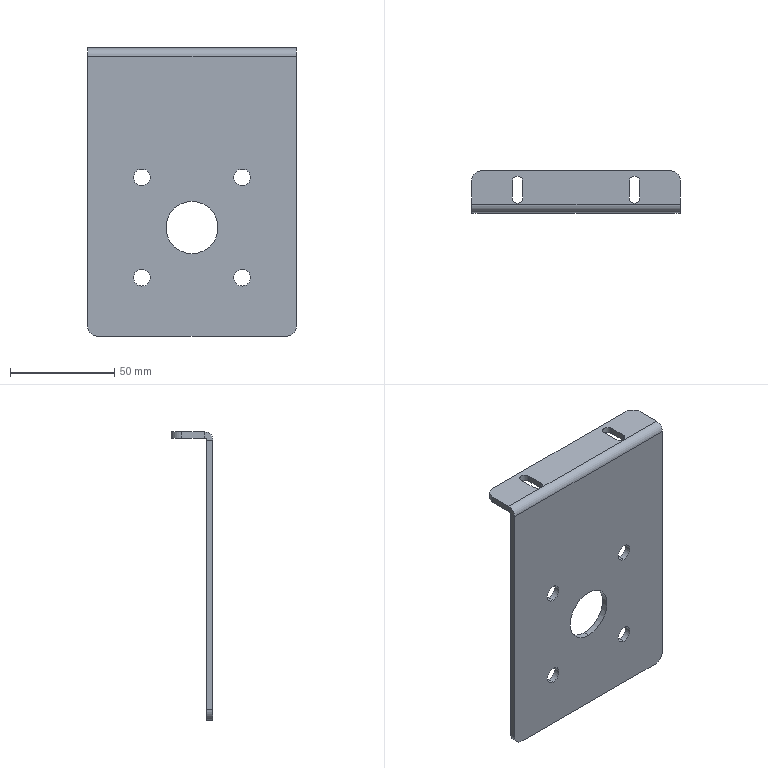Part | STEP file | 11-FG-JX00511 | 1 solid | 36 faces | box 100 x 20 x 138 mm | volume 43680 mm3 | cylinder 20 | plane 16 | commonest cylinder face diameters 8 x9 5 x4 10 x4 25 x2 2 x1
STEP:
#1=CARTESIAN_POINT('',(-24.,-10.,-66.));
#2=VERTEX_POINT('',#1);
#3=CARTESIAN_POINT('',(-24.,-10.,-58.));
#4=VERTEX_POINT('',#3);
#5=CARTESIAN_POINT('',(-24.,-10.,-62.));
#6=DIRECTION('',(0.,1.,0.));
#7=DIRECTION('',(0.,0.,1.));
#8=AXIS2_PLACEMENT_3D('',#5,#6,#7);
#9=CIRCLE('',#8,4.);
#10=EDGE_CURVE('',#2,#4,#9,.T.);
#11=ORIENTED_EDGE('',*,*,#10,.F.);
#12=CARTESIAN_POINT('',(-24.,-7.,-66.));
#13=VERTEX_POINT('',#12);
#14=CARTESIAN_POINT('',(-24.,-10.,-66.));
#15=DIRECTION('',(0.,1.,0.));
#16=VECTOR('',#15,1000.);
#17=LINE('',#14,#16);
#18=EDGE_CURVE('',#2,#13,#17,.T.);
#19=ORIENTED_EDGE('',*,*,#18,.T.);
#20=CARTESIAN_POINT('',(-24.,-7.,-58.));
#21=VERTEX_POINT('',#20);
#22=CARTESIAN_POINT('',(-24.,-7.,-62.));
#23=DIRECTION('',(0.,1.,0.));
#24=DIRECTION('',(0.,0.,1.));
#25=AXIS2_PLACEMENT_3D('',#22,#23,#24);
#26=CIRCLE('',#25,4.);
#27=EDGE_CURVE('',#13,#21,#26,.T.);
#28=ORIENTED_EDGE('',*,*,#27,.T.);
#29=CARTESIAN_POINT('',(-24.,-10.,-58.));
#30=DIRECTION('',(0.,1.,0.));
#31=VECTOR('',#30,1000.);
#32=LINE('',#29,#31);
#33=EDGE_CURVE('',#4,#21,#32,.T.);
#34=ORIENTED_EDGE('',*,*,#33,.F.);
#35=EDGE_LOOP('',(#11,#19,#28,#34));
#36=FACE_OUTER_BOUND('',#35,.T.);
#37=CARTESIAN_POINT('',(-24.,-10.,-62.));
#38=DIRECTION('',(0.,1.,0.));
#39=DIRECTION('',(0.,0.,1.));
#40=AXIS2_PLACEMENT_3D('',#37,#38,#39);
#41=CYLINDRICAL_SURFACE('',#40,4.);
#42=ADVANCED_FACE('',(#36),#41,.F.);
#43=CARTESIAN_POINT('',(-24.,-10.,-114.));
#44=VERTEX_POINT('',#43);
#45=CARTESIAN_POINT('',(-24.,-10.,-106.));
#46=VERTEX_POINT('',#45);
#47=CARTESIAN_POINT('',(-24.,-10.,-110.));
#48=DIRECTION('',(0.,1.,0.));
#49=DIRECTION('',(0.,0.,1.));
#50=AXIS2_PLACEMENT_3D('',#47,#48,#49);
#51=CIRCLE('',#50,4.);
#52=EDGE_CURVE('',#44,#46,#51,.T.);
#53=ORIENTED_EDGE('',*,*,#52,.F.);
#54=CARTESIAN_POINT('',(-24.,-7.,-114.));
#55=VERTEX_POINT('',#54);
#56=CARTESIAN_POINT('',(-24.,-10.,-114.));
#57=DIRECTION('',(0.,1.,0.));
#58=VECTOR('',#57,1000.);
#59=LINE('',#56,#58);
#60=EDGE_CURVE('',#44,#55,#59,.T.);
#61=ORIENTED_EDGE('',*,*,#60,.T.);
#62=CARTESIAN_POINT('',(-24.,-7.,-106.));
#63=VERTEX_POINT('',#62);
#64=CARTESIAN_POINT('',(-24.,-7.,-110.));
#65=DIRECTION('',(0.,1.,0.));
#66=DIRECTION('',(0.,0.,1.));
#67=AXIS2_PLACEMENT_3D('',#64,#65,#66);
#68=CIRCLE('',#67,4.);
#69=EDGE_CURVE('',#55,#63,#68,.T.);
#70=ORIENTED_EDGE('',*,*,#69,.T.);
#71=CARTESIAN_POINT('',(-24.,-10.,-106.));
#72=DIRECTION('',(0.,1.,0.));
#73=VECTOR('',#72,1000.);
#74=LINE('',#71,#73);
#75=EDGE_CURVE('',#46,#63,#74,.T.);
#76=ORIENTED_EDGE('',*,*,#75,.F.);
#77=EDGE_LOOP('',(#53,#61,#70,#76));
#78=FACE_OUTER_BOUND('',#77,.T.);
#79=CARTESIAN_POINT('',(-24.,-10.,-110.));
#80=DIRECTION('',(0.,1.,0.));
#81=DIRECTION('',(0.,0.,1.));
#82=AXIS2_PLACEMENT_3D('',#79,#80,#81);
#83=CYLINDRICAL_SURFACE('',#82,4.);
#84=ADVANCED_FACE('',(#78),#83,.F.);
#85=CARTESIAN_POINT('',(24.,-10.,-114.));
#86=VERTEX_POINT('',#85);
#87=CARTESIAN_POINT('',(24.,-10.,-106.));
#88=VERTEX_POINT('',#87);
#89=CARTESIAN_POINT('',(24.,-10.,-110.));
#90=DIRECTION('',(0.,1.,0.));
#91=DIRECTION('',(0.,0.,1.));
#92=AXIS2_PLACEMENT_3D('',#89,#90,#91);
#93=CIRCLE('',#92,4.);
#94=EDGE_CURVE('',#86,#88,#93,.T.);
#95=ORIENTED_EDGE('',*,*,#94,.F.);
#96=CARTESIAN_POINT('',(24.,-7.,-114.));
#97=VERTEX_POINT('',#96);
#98=CARTESIAN_POINT('',(24.,-10.,-114.));
#99=DIRECTION('',(0.,1.,0.));
#100=VECTOR('',#99,1000.);
#101=LINE('',#98,#100);
#102=EDGE_CURVE('',#86,#97,#101,.T.);
#103=ORIENTED_EDGE('',*,*,#102,.T.);
#104=CARTESIAN_POINT('',(24.,-7.,-106.));
#105=VERTEX_POINT('',#104);
#106=CARTESIAN_POINT('',(24.,-7.,-110.));
#107=DIRECTION('',(0.,1.,0.));
#108=DIRECTION('',(0.,0.,1.));
#109=AXIS2_PLACEMENT_3D('',#106,#107,#108);
#110=CIRCLE('',#109,4.);
#111=EDGE_CURVE('',#97,#105,#110,.T.);
#112=ORIENTED_EDGE('',*,*,#111,.T.);
#113=CARTESIAN_POINT('',(24.,-10.,-106.));
#114=DIRECTION('',(0.,1.,0.));
#115=VECTOR('',#114,1000.);
#116=LINE('',#113,#115);
#117=EDGE_CURVE('',#88,#105,#116,.T.);
#118=ORIENTED_EDGE('',*,*,#117,.F.);
#119=EDGE_LOOP('',(#95,#103,#112,#118));
#120=FACE_OUTER_BOUND('',#119,.T.);
#121=CARTESIAN_POINT('',(24.,-10.,-110.));
#122=DIRECTION('',(0.,1.,0.));
#123=DIRECTION('',(0.,0.,1.));
#124=AXIS2_PLACEMENT_3D('',#121,#122,#123);
#125=CYLINDRICAL_SURFACE('',#124,4.);
#126=ADVANCED_FACE('',(#120),#125,.F.);
#127=CARTESIAN_POINT('',(24.,-10.,-66.));
#128=VERTEX_POINT('',#127);
#129=CARTESIAN_POINT('',(24.,-10.,-58.));
#130=VERTEX_POINT('',#129);
#131=CARTESIAN_POINT('',(24.,-10.,-62.));
#132=DIRECTION('',(0.,1.,0.));
#133=DIRECTION('',(0.,0.,1.));
#134=AXIS2_PLACEMENT_3D('',#131,#132,#133);
#135=CIRCLE('',#134,4.);
#136=EDGE_CURVE('',#128,#130,#135,.T.);
#137=ORIENTED_EDGE('',*,*,#136,.F.);
#138=CARTESIAN_POINT('',(24.,-7.,-66.));
#139=VERTEX_POINT('',#138);
#140=CARTESIAN_POINT('',(24.,-10.,-66.));
#141=DIRECTION('',(0.,1.,0.));
#142=VECTOR('',#141,1000.);
#143=LINE('',#140,#142);
#144=EDGE_CURVE('',#128,#139,#143,.T.);
#145=ORIENTED_EDGE('',*,*,#144,.T.);
#146=CARTESIAN_POINT('',(24.,-7.,-58.));
#147=VERTEX_POINT('',#146);
#148=CARTESIAN_POINT('',(24.,-7.,-62.));
#149=DIRECTION('',(0.,1.,0.));
#150=DIRECTION('',(0.,0.,1.));
#151=AXIS2_PLACEMENT_3D('',#148,#149,#150);
#152=CIRCLE('',#151,4.);
#153=EDGE_CURVE('',#139,#147,#152,.T.);
#154=ORIENTED_EDGE('',*,*,#153,.T.);
#155=CARTESIAN_POINT('',(24.,-10.,-58.));
#156=DIRECTION('',(0.,1.,0.));
#157=VECTOR('',#156,1000.);
#158=LINE('',#155,#157);
#159=EDGE_CURVE('',#130,#147,#158,.T.);
#160=ORIENTED_EDGE('',*,*,#159,.F.);
#161=EDGE_LOOP('',(#137,#145,#154,#160));
#162=FACE_OUTER_BOUND('',#161,.T.);
#163=CARTESIAN_POINT('',(24.,-10.,-62.));
#164=DIRECTION('',(0.,1.,0.));
#165=DIRECTION('',(0.,0.,1.));
#166=AXIS2_PLACEMENT_3D('',#163,#164,#165);
#167=CYLINDRICAL_SURFACE('',#166,4.);
#168=ADVANCED_FACE('',(#162),#167,.F.);
#169=CARTESIAN_POINT('',(0.,-10.,-98.5));
#170=VERTEX_POINT('',#169);
#171=CARTESIAN_POINT('',(0.,-10.,-73.5));
#172=VERTEX_POINT('',#171);
#173=CARTESIAN_POINT('',(0.,-10.,-86.));
#174=DIRECTION('',(0.,1.,0.));
#175=DIRECTION('',(0.,0.,1.));
#176=AXIS2_PLACEMENT_3D('',#173,#174,#175);
#177=CIRCLE('',#176,12.5);
#178=EDGE_CURVE('',#170,#172,#177,.T.);
#179=ORIENTED_EDGE('',*,*,#178,.F.);
#180=CARTESIAN_POINT('',(0.,-7.,-98.5));
#181=VERTEX_POINT('',#180);
#182=CARTESIAN_POINT('',(0.,-10.,-98.5));
#183=DIRECTION('',(0.,1.,0.));
#184=VECTOR('',#183,1000.);
#185=LINE('',#182,#184);
#186=EDGE_CURVE('',#170,#181,#185,.T.);
#187=ORIENTED_EDGE('',*,*,#186,.T.);
#188=CARTESIAN_POINT('',(0.,-7.,-73.5));
#189=VERTEX_POINT('',#188);
#190=CARTESIAN_POINT('',(0.,-7.,-86.));
#191=DIRECTION('',(0.,1.,0.));
#192=DIRECTION('',(0.,0.,1.));
#193=AXIS2_PLACEMENT_3D('',#190,#191,#192);
#194=CIRCLE('',#193,12.5);
#195=EDGE_CURVE('',#181,#189,#194,.T.);
#196=ORIENTED_EDGE('',*,*,#195,.T.);
#197=CARTESIAN_POINT('',(0.,-10.,-73.5));
#198=DIRECTION('',(0.,1.,0.));
#199=VECTOR('',#198,1000.);
#200=LINE('',#197,#199);
#201=EDGE_CURVE('',#172,#189,#200,.T.);
#202=ORIENTED_EDGE('',*,*,#201,.F.);
#203=EDGE_LOOP('',(#179,#187,#196,#202));
#204=FACE_OUTER_BOUND('',#203,.T.);
#205=CARTESIAN_POINT('',(0.,-10.,-86.));
#206=DIRECTION('',(0.,1.,0.));
#207=DIRECTION('',(0.,0.,1.));
#208=AXIS2_PLACEMENT_3D('',#205,#206,#207);
#209=CYLINDRICAL_SURFACE('',#208,12.5);
#210=ADVANCED_FACE('',(#204),#209,.F.);
#211=CARTESIAN_POINT('',(-50.,5.,0.));
#212=VERTEX_POINT('',#211);
#213=CARTESIAN_POINT('',(-50.,-6.,0.));
#214=VERTEX_POINT('',#213);
#215=CARTESIAN_POINT('',(-50.,10.,0.));
#216=DIRECTION('',(0.,-1.,0.));
#217=VECTOR('',#216,1000.);
#218=LINE('',#215,#217);
#219=EDGE_CURVE('',#212,#214,#218,.T.);
#220=ORIENTED_EDGE('',*,*,#219,.F.);
#221=CARTESIAN_POINT('',(-50.,5.,-3.));
#222=VERTEX_POINT('',#221);
#223=CARTESIAN_POINT('',(-50.,5.,-3.));
#224=DIRECTION('',(0.,0.,-1.));
#225=VECTOR('',#224,1000.);
#226=LINE('',#223,#225);
#227=EDGE_CURVE('',#212,#222,#226,.T.);
#228=ORIENTED_EDGE('',*,*,#227,.T.);
#229=CARTESIAN_POINT('',(-50.,-6.,-3.));
#230=VERTEX_POINT('',#229);
#231=CARTESIAN_POINT('',(-50.,10.,-3.));
#232=DIRECTION('',(0.,-1.,0.));
#233=VECTOR('',#232,1000.);
#234=LINE('',#231,#233);
#235=EDGE_CURVE('',#222,#230,#234,.T.);
#236=ORIENTED_EDGE('',*,*,#235,.T.);
#237=CARTESIAN_POINT('',(-50.,-6.,-3.));
#238=DIRECTION('',(0.,0.,1.));
#239=VECTOR('',#238,1000.);
#240=LINE('',#237,#239);
#241=EDGE_CURVE('',#230,#214,#240,.T.);
#242=ORIENTED_EDGE('',*,*,#241,.T.);
#243=EDGE_LOOP('',(#220,#228,#236,#242));
#244=FACE_OUTER_BOUND('',#243,.T.);
#245=CARTESIAN_POINT('',(-50.,10.,-3.));
#246=DIRECTION('',(-1.,0.,0.));
#247=DIRECTION('',(0.,0.,1.));
#248=AXIS2_PLACEMENT_3D('',#245,#246,#247);
#249=PLANE('',#248);
#250=ADVANCED_FACE('',(#244),#249,.T.);
#251=CARTESIAN_POINT('',(30.5,5.,-3.));
#252=VERTEX_POINT('',#251);
#253=CARTESIAN_POINT('',(30.5,-3.,-3.));
#254=VERTEX_POINT('',#253);
#255=CARTESIAN_POINT('',(30.5,5.,-3.));
#256=DIRECTION('',(0.,-1.,0.));
#257=VECTOR('',#256,1000.);
#258=LINE('',#255,#257);
#259=EDGE_CURVE('',#252,#254,#258,.T.);
#260=ORIENTED_EDGE('',*,*,#259,.F.);
#261=CARTESIAN_POINT('',(25.5,5.,-3.));
#262=VERTEX_POINT('',#261);
#263=CARTESIAN_POINT('',(28.,5.,-3.));
#264=DIRECTION('',(0.,0.,-1.));
#265=DIRECTION('',(1.,0.,0.));
#266=AXIS2_PLACEMENT_3D('',#263,#264,#265);
#267=CIRCLE('',#266,2.5);
#268=EDGE_CURVE('',#262,#252,#267,.T.);
#269=ORIENTED_EDGE('',*,*,#268,.F.);
#270=CARTESIAN_POINT('',(25.5,-3.,-3.));
#271=VERTEX_POINT('',#270);
#272=CARTESIAN_POINT('',(25.5,5.,-3.));
#273=DIRECTION('',(0.,1.,0.));
#274=VECTOR('',#273,1000.);
#275=LINE('',#272,#274);
#276=EDGE_CURVE('',#271,#262,#275,.T.);
#277=ORIENTED_EDGE('',*,*,#276,.F.);
#278=CARTESIAN_POINT('',(28.,-3.,-3.));
#279=DIRECTION('',(0.,0.,-1.));
#280=DIRECTION('',(1.,0.,0.));
#281=AXIS2_PLACEMENT_3D('',#278,#279,#280);
#282=CIRCLE('',#281,2.5);
#283=EDGE_CURVE('',#254,#271,#282,.T.);
#284=ORIENTED_EDGE('',*,*,#283,.F.);
#285=EDGE_LOOP('',(#260,#269,#277,#284));
#286=FACE_BOUND('',#285,.T.);
#287=CARTESIAN_POINT('',(-25.5,5.,-3.));
#288=VERTEX_POINT('',#287);
#289=CARTESIAN_POINT('',(-25.5,-3.,-3.));
#290=VERTEX_POINT('',#289);
#291=CARTESIAN_POINT('',(-25.5,5.,-3.));
#292=DIRECTION('',(0.,-1.,0.));
#293=VECTOR('',#292,1000.);
#294=LINE('',#291,#293);
#295=EDGE_CURVE('',#288,#290,#294,.T.);
#296=ORIENTED_EDGE('',*,*,#295,.F.);
#297=CARTESIAN_POINT('',(-30.5,5.,-3.));
#298=VERTEX_POINT('',#297);
#299=CARTESIAN_POINT('',(-28.,5.,-3.));
#300=DIRECTION('',(0.,0.,-1.));
#301=DIRECTION('',(-1.,0.,0.));
#302=AXIS2_PLACEMENT_3D('',#299,#300,#301);
#303=CIRCLE('',#302,2.5);
#304=EDGE_CURVE('',#298,#288,#303,.T.);
#305=ORIENTED_EDGE('',*,*,#304,.F.);
#306=CARTESIAN_POINT('',(-30.5,-3.,-3.));
#307=VERTEX_POINT('',#306);
#308=CARTESIAN_POINT('',(-30.5,5.,-3.));
#309=DIRECTION('',(0.,1.,0.));
#310=VECTOR('',#309,1000.);
#311=LINE('',#308,#310);
#312=EDGE_CURVE('',#307,#298,#311,.T.);
#313=ORIENTED_EDGE('',*,*,#312,.F.);
#314=CARTESIAN_POINT('',(-28.,-3.,-3.));
#315=DIRECTION('',(0.,0.,-1.));
#316=DIRECTION('',(-1.,0.,0.));
#317=AXIS2_PLACEMENT_3D('',#314,#315,#316);
#318=CIRCLE('',#317,2.5);
#319=EDGE_CURVE('',#290,#307,#318,.T.);
#320=ORIENTED_EDGE('',*,*,#319,.F.);
#321=EDGE_LOOP('',(#296,#305,#313,#320));
#322=FACE_BOUND('',#321,.T.);
#323=CARTESIAN_POINT('',(45.,10.,-3.));
#324=VERTEX_POINT('',#323);
#325=CARTESIAN_POINT('',(-45.,10.,-3.));
#326=VERTEX_POINT('',#325);
#327=CARTESIAN_POINT('',(-50.,10.,-3.));
#328=DIRECTION('',(-1.,0.,0.));
#329=VECTOR('',#328,1000.);
#330=LINE('',#327,#329);
#331=EDGE_CURVE('',#324,#326,#330,.T.);
#332=ORIENTED_EDGE('',*,*,#331,.F.);
#333=CARTESIAN_POINT('',(50.,5.,-3.));
#334=VERTEX_POINT('',#333);
#335=CARTESIAN_POINT('',(45.,5.,-3.));
#336=DIRECTION('',(0.,0.,-1.));
#337=DIRECTION('',(1.,0.,0.));
#338=AXIS2_PLACEMENT_3D('',#335,#336,#337);
#339=CIRCLE('',#338,5.);
#340=EDGE_CURVE('',#324,#334,#339,.T.);
#341=ORIENTED_EDGE('',*,*,#340,.T.);
#342=CARTESIAN_POINT('',(50.,-6.,-3.));
#343=VERTEX_POINT('',#342);
#344=CARTESIAN_POINT('',(50.,10.,-3.));
#345=DIRECTION('',(0.,1.,0.));
#346=VECTOR('',#345,1000.);
#347=LINE('',#344,#346);
#348=EDGE_CURVE('',#343,#334,#347,.T.);
#349=ORIENTED_EDGE('',*,*,#348,.F.);
#350=CARTESIAN_POINT('',(-50.,-6.,-3.));
#351=DIRECTION('',(1.,0.,0.));
#352=VECTOR('',#351,1000.);
#353=LINE('',#350,#352);
#354=EDGE_CURVE('',#230,#343,#353,.T.);
#355=ORIENTED_EDGE('',*,*,#354,.F.);
#356=ORIENTED_EDGE('',*,*,#235,.F.);
#357=CARTESIAN_POINT('',(-45.,5.,-3.));
#358=DIRECTION('',(0.,0.,-1.));
#359=DIRECTION('',(1.,0.,0.));
#360=AXIS2_PLACEMENT_3D('',#357,#358,#359);
#361=CIRCLE('',#360,5.);
#362=EDGE_CURVE('',#222,#326,#361,.T.);
#363=ORIENTED_EDGE('',*,*,#362,.T.);
#364=EDGE_LOOP('',(#332,#341,#349,#355,#356,#363));
#365=FACE_OUTER_BOUND('',#364,.T.);
#366=CARTESIAN_POINT('',(0.,0.,-3.));
#367=DIRECTION('',(0.,0.,1.));
#368=DIRECTION('',(1.,0.,0.));
#369=AXIS2_PLACEMENT_3D('',#366,#367,#368);
#370=PLANE('',#369);
#371=ADVANCED_FACE('',(#286,#322,#365),#370,.F.);
#372=CARTESIAN_POINT('',(25.5,5.,0.));
#373=VERTEX_POINT('',#372);
#374=CARTESIAN_POINT('',(30.5,5.,0.));
#375=VERTEX_POINT('',#374);
#376=CARTESIAN_POINT('',(28.,5.,0.));
#377=DIRECTION('',(0.,0.,-1.));
#378=DIRECTION('',(1.,0.,0.));
#379=AXIS2_PLACEMENT_3D('',#376,#377,#378);
#380=CIRCLE('',#379,2.5);
#381=EDGE_CURVE('',#373,#375,#380,.T.);
#382=ORIENTED_EDGE('',*,*,#381,.T.);
#383=CARTESIAN_POINT('',(30.5,-3.,0.));
#384=VERTEX_POINT('',#383);
#385=CARTESIAN_POINT('',(30.5,5.,0.));
#386=DIRECTION('',(0.,-1.,0.));
#387=VECTOR('',#386,1000.);
#388=LINE('',#385,#387);
#389=EDGE_CURVE('',#375,#384,#388,.T.);
#390=ORIENTED_EDGE('',*,*,#389,.T.);
#391=CARTESIAN_POINT('',(25.5,-3.,0.));
#392=VERTEX_POINT('',#391);
#393=CARTESIAN_POINT('',(28.,-3.,0.));
#394=DIRECTION('',(0.,0.,-1.));
#395=DIRECTION('',(1.,0.,0.));
#396=AXIS2_PLACEMENT_3D('',#393,#394,#395);
#397=CIRCLE('',#396,2.5);
#398=EDGE_CURVE('',#384,#392,#397,.T.);
#399=ORIENTED_EDGE('',*,*,#398,.T.);
#400=CARTESIAN_POINT('',(25.5,5.,0.));
#401=DIRECTION('',(0.,1.,0.));
#402=VECTOR('',#401,1000.);
#403=LINE('',#400,#402);
#404=EDGE_CURVE('',#392,#373,#403,.T.);
#405=ORIENTED_EDGE('',*,*,#404,.T.);
#406=EDGE_LOOP('',(#382,#390,#399,#405));
#407=FACE_BOUND('',#406,.T.);
#408=CARTESIAN_POINT('',(-30.5,5.,0.));
#409=VERTEX_POINT('',#408);
#410=CARTESIAN_POINT('',(-25.5,5.,0.));
#411=VERTEX_POINT('',#410);
#412=CARTESIAN_POINT('',(-28.,5.,0.));
#413=DIRECTION('',(0.,0.,-1.));
#414=DIRECTION('',(-1.,0.,0.));
#415=AXIS2_PLACEMENT_3D('',#412,#413,#414);
#416=CIRCLE('',#415,2.5);
#417=EDGE_CURVE('',#409,#411,#416,.T.);
#418=ORIENTED_EDGE('',*,*,#417,.T.);
#419=CARTESIAN_POINT('',(-25.5,-3.,0.));
#420=VERTEX_POINT('',#419);
#421=CARTESIAN_POINT('',(-25.5,5.,0.));
#422=DIRECTION('',(0.,-1.,0.));
#423=VECTOR('',#422,1000.);
#424=LINE('',#421,#423);
#425=EDGE_CURVE('',#411,#420,#424,.T.);
#426=ORIENTED_EDGE('',*,*,#425,.T.);
#427=CARTESIAN_POINT('',(-30.5,-3.,0.));
#428=VERTEX_POINT('',#427);
#429=CARTESIAN_POINT('',(-28.,-3.,0.));
#430=DIRECTION('',(0.,0.,-1.));
#431=DIRECTION('',(-1.,0.,0.));
#432=AXIS2_PLACEMENT_3D('',#429,#430,#431);
#433=CIRCLE('',#432,2.5);
#434=EDGE_CURVE('',#420,#428,#433,.T.);
#435=ORIENTED_EDGE('',*,*,#434,.T.);
#436=CARTESIAN_POINT('',(-30.5,5.,0.));
#437=DIRECTION('',(0.,1.,0.));
#438=VECTOR('',#437,1000.);
#439=LINE('',#436,#438);
#440=EDGE_CURVE('',#428,#409,#439,.T.);
#441=ORIENTED_EDGE('',*,*,#440,.T.);
#442=EDGE_LOOP('',(#418,#426,#435,#441));
#443=FACE_BOUND('',#442,.T.);
#444=CARTESIAN_POINT('',(50.,-6.,0.));
#445=VERTEX_POINT('',#444);
#446=CARTESIAN_POINT('',(50.,5.,0.));
#447=VERTEX_POINT('',#446);
#448=CARTESIAN_POINT('',(50.,10.,0.));
#449=DIRECTION('',(0.,1.,0.));
#450=VECTOR('',#449,1000.);
#451=LINE('',#448,#450);
#452=EDGE_CURVE('',#445,#447,#451,.T.);
#453=ORIENTED_EDGE('',*,*,#452,.T.);
#454=CARTESIAN_POINT('',(45.,10.,0.));
#455=VERTEX_POINT('',#454);
#456=CARTESIAN_POINT('',(45.,5.,0.));
#457=DIRECTION('',(0.,0.,1.));
#458=DIRECTION('',(1.,0.,0.));
#459=AXIS2_PLACEMENT_3D('',#456,#457,#458);
#460=CIRCLE('',#459,5.);
#461=EDGE_CURVE('',#447,#455,#460,.T.);
#462=ORIENTED_EDGE('',*,*,#461,.T.);
#463=CARTESIAN_POINT('',(-45.,10.,0.));
#464=VERTEX_POINT('',#463);
#465=CARTESIAN_POINT('',(-50.,10.,0.));
#466=DIRECTION('',(-1.,0.,0.));
#467=VECTOR('',#466,1000.);
#468=LINE('',#465,#467);
#469=EDGE_CURVE('',#455,#464,#468,.T.);
#470=ORIENTED_EDGE('',*,*,#469,.T.);
#471=CARTESIAN_POINT('',(-45.,5.,0.));
#472=DIRECTION('',(0.,0.,1.));
#473=DIRECTION('',(1.,0.,0.));
#474=AXIS2_PLACEMENT_3D('',#471,#472,#473);
#475=CIRCLE('',#474,5.);
#476=EDGE_CURVE('',#464,#212,#475,.T.);
#477=ORIENTED_EDGE('',*,*,#476,.T.);
#478=ORIENTED_EDGE('',*,*,#219,.T.);
#479=CARTESIAN_POINT('',(-50.,-6.,0.));
#480=DIRECTION('',(1.,0.,0.));
#481=VECTOR('',#480,1000.);
#482=LINE('',#479,#481);
#483=EDGE_CURVE('',#214,#445,#482,.T.);
#484=ORIENTED_EDGE('',*,*,#483,.T.);
#485=EDGE_LOOP('',(#453,#462,#470,#477,#478,#484));
#486=FACE_OUTER_BOUND('',#485,.T.);
#487=CARTESIAN_POINT('',(0.,0.,0.));
#488=DIRECTION('',(0.,0.,1.));
#489=DIRECTION('',(1.,0.,0.));
#490=AXIS2_PLACEMENT_3D('',#487,#488,#489);
#491=PLANE('',#490);
#492=ADVANCED_FACE('',(#407,#443,#486),#491,.T.);
#493=ORIENTED_EDGE('',*,*,#348,.T.);
#494=CARTESIAN_POINT('',(50.,5.,-3.));
#495=DIRECTION('',(0.,0.,1.));
#496=VECTOR('',#495,1000.);
#497=LINE('',#494,#496);
#498=EDGE_CURVE('',#334,#447,#497,.T.);
#499=ORIENTED_EDGE('',*,*,#498,.T.);
#500=ORIENTED_EDGE('',*,*,#452,.F.);
#501=CARTESIAN_POINT('',(50.,-6.,-3.));
#502=DIRECTION('',(0.,0.,1.));
#503=VECTOR('',#502,1000.);
#504=LINE('',#501,#503);
#505=EDGE_CURVE('',#343,#445,#504,.T.);
#506=ORIENTED_EDGE('',*,*,#505,.F.);
#507=EDGE_LOOP('',(#493,#499,#500,#506));
#508=FACE_OUTER_BOUND('',#507,.T.);
#509=CARTESIAN_POINT('',(50.,10.,-3.));
#510=DIRECTION('',(1.,0.,0.));
#511=DIRECTION('',(0.,1.,0.));
#512=AXIS2_PLACEMENT_3D('',#509,#510,#511);
#513=PLANE('',#512);
#514=ADVANCED_FACE('',(#508),#513,.T.);
#515=ORIENTED_EDGE('',*,*,#469,.F.);
#516=CARTESIAN_POINT('',(45.,10.,-3.));
#517=DIRECTION('',(0.,0.,-1.));
#518=VECTOR('',#517,1000.);
#519=LINE('',#516,#518);
#520=EDGE_CURVE('',#455,#324,#519,.T.);
#521=ORIENTED_EDGE('',*,*,#520,.T.);
#522=ORIENTED_EDGE('',*,*,#331,.T.);
#523=CARTESIAN_POINT('',(-45.,10.,-3.));
#524=DIRECTION('',(0.,0.,1.));
#525=VECTOR('',#524,1000.);
#526=LINE('',#523,#525);
#527=EDGE_CURVE('',#326,#464,#526,.T.);
#528=ORIENTED_EDGE('',*,*,#527,.T.);
#529=EDGE_LOOP('',(#515,#521,#522,#528));
#530=FACE_OUTER_BOUND('',#529,.T.);
#531=CARTESIAN_POINT('',(-50.,10.,-3.));
#532=DIRECTION('',(0.,1.,0.));
#533=DIRECTION('',(0.,0.,1.));
#534=AXIS2_PLACEMENT_3D('',#531,#532,#533);
#535=PLANE('',#534);
#536=ADVANCED_FACE('',(#530),#535,.T.);
#537=CARTESIAN_POINT('',(50.,-7.,-4.));
#538=VERTEX_POINT('',#537);
#539=CARTESIAN_POINT('',(50.,-10.,-4.));
#540=VERTEX_POINT('',#539);
#541=CARTESIAN_POINT('',(50.,-10.,-4.));
#542=DIRECTION('',(0.,-1.,0.));
#543=VECTOR('',#542,1000.);
#544=LINE('',#541,#543);
#545=EDGE_CURVE('',#538,#540,#544,.T.);
#546=ORIENTED_EDGE('',*,*,#545,.F.);
#547=CARTESIAN_POINT('',(50.,-6.,-4.));
#548=DIRECTION('',(1.,0.,0.));
#549=DIRECTION('',(0.,0.,1.));
#550=AXIS2_PLACEMENT_3D('',#547,#548,#549);
#551=CIRCLE('',#550,1.);
#552=EDGE_CURVE('',#343,#538,#551,.T.);
#553=ORIENTED_EDGE('',*,*,#552,.F.);
#554=ORIENTED_EDGE('',*,*,#505,.T.);
#555=CARTESIAN_POINT('',(50.,-6.,-4.));
#556=DIRECTION('',(1.,0.,0.));
#557=DIRECTION('',(0.,0.,1.));
#558=AXIS2_PLACEMENT_3D('',#555,#556,#557);
#559=CIRCLE('',#558,4.);
#560=EDGE_CURVE('',#445,#540,#559,.T.);
#561=ORIENTED_EDGE('',*,*,#560,.T.);
#562=EDGE_LOOP('',(#546,#553,#554,#561));
#563=FACE_OUTER_BOUND('',#562,.T.);
#564=CARTESIAN_POINT('',(50.,-6.,-4.));
#565=DIRECTION('',(1.,0.,0.));
#566=DIRECTION('',(0.,0.,-1.));
#567=AXIS2_PLACEMENT_3D('',#564,#565,#566);
#568=PLANE('',#567);
#569=ADVANCED_FACE('',(#563),#568,.T.);
#570=CARTESIAN_POINT('',(-50.,-7.,-4.));
#571=VERTEX_POINT('',#570);
#572=CARTESIAN_POINT('',(-50.,-6.,-4.));
#573=DIRECTION('',(-1.,0.,0.));
#574=DIRECTION('',(0.,0.,1.));
#575=AXIS2_PLACEMENT_3D('',#572,#573,#574);
#576=CIRCLE('',#575,1.);
#577=EDGE_CURVE('',#571,#230,#576,.T.);
#578=ORIENTED_EDGE('',*,*,#577,.F.);
#579=CARTESIAN_POINT('',(-50.,-10.,-4.));
#580=VERTEX_POINT('',#579);
#581=CARTESIAN_POINT('',(-50.,-7.,-4.));
#582=DIRECTION('',(0.,-1.,0.));
#583=VECTOR('',#582,1000.);
#584=LINE('',#581,#583);
#585=EDGE_CURVE('',#571,#580,#584,.T.);
#586=ORIENTED_EDGE('',*,*,#585,.T.);
#587=CARTESIAN_POINT('',(-50.,-6.,-4.));
#588=DIRECTION('',(-1.,0.,0.));
#589=DIRECTION('',(0.,0.,1.));
#590=AXIS2_PLACEMENT_3D('',#587,#588,#589);
#591=CIRCLE('',#590,4.);
#592=EDGE_CURVE('',#580,#214,#591,.T.);
#593=ORIENTED_EDGE('',*,*,#592,.T.);
#594=ORIENTED_EDGE('',*,*,#241,.F.);
#595=EDGE_LOOP('',(#578,#586,#593,#594));
#596=FACE_OUTER_BOUND('',#595,.T.);
#597=CARTESIAN_POINT('',(-50.,-6.,-4.));
#598=DIRECTION('',(1.,0.,0.));
#599=DIRECTION('',(0.,0.,-1.));
#600=AXIS2_PLACEMENT_3D('',#597,#598,#599);
#601=PLANE('',#600);
#602=ADVANCED_FACE('',(#596),#601,.F.);
#603=ORIENTED_EDGE('',*,*,#483,.F.);
#604=ORIENTED_EDGE('',*,*,#592,.F.);
#605=CARTESIAN_POINT('',(50.,-10.,-4.));
#606=DIRECTION('',(1.,0.,0.));
#607=VECTOR('',#606,1000.);
#608=LINE('',#605,#607);
#609=EDGE_CURVE('',#580,#540,#608,.T.);
#610=ORIENTED_EDGE('',*,*,#609,.T.);
#611=ORIENTED_EDGE('',*,*,#560,.F.);
#612=EDGE_LOOP('',(#603,#604,#610,#611));
#613=FACE_OUTER_BOUND('',#612,.T.);
#614=CARTESIAN_POINT('',(-50.,-6.,-4.));
#615=DIRECTION('',(-1.,0.,0.));
#616=DIRECTION('',(0.,-1.,0.));
#617=AXIS2_PLACEMENT_3D('',#614,#615,#616);
#618=CYLINDRICAL_SURFACE('',#617,4.);
#619=ADVANCED_FACE('',(#613),#618,.T.);
#620=ORIENTED_EDGE('',*,*,#354,.T.);
#621=ORIENTED_EDGE('',*,*,#552,.T.);
#622=CARTESIAN_POINT('',(50.,-7.,-4.));
#623=DIRECTION('',(-1.,0.,0.));
#624=VECTOR('',#623,1000.);
#625=LINE('',#622,#624);
#626=EDGE_CURVE('',#538,#571,#625,.T.);
#627=ORIENTED_EDGE('',*,*,#626,.T.);
#628=ORIENTED_EDGE('',*,*,#577,.T.);
#629=EDGE_LOOP('',(#620,#621,#627,#628));
#630=FACE_OUTER_BOUND('',#629,.T.);
#631=CARTESIAN_POINT('',(-50.,-6.,-4.));
#632=DIRECTION('',(-1.,0.,0.));
#633=DIRECTION('',(0.,-1.,0.));
#634=AXIS2_PLACEMENT_3D('',#631,#632,#633);
#635=CYLINDRICAL_SURFACE('',#634,1.);
#636=ADVANCED_FACE('',(#630),#635,.F.);
#637=CARTESIAN_POINT('',(-50.,-7.,-133.));
#638=VERTEX_POINT('',#637);
#639=CARTESIAN_POINT('',(-50.,-7.,-138.));
#640=DIRECTION('',(0.,0.,-1.));
#641=VECTOR('',#640,1000.);
#642=LINE('',#639,#641);
#643=EDGE_CURVE('',#571,#638,#642,.T.);
#644=ORIENTED_EDGE('',*,*,#643,.T.);
#645=CARTESIAN_POINT('',(-50.,-10.,-133.));
#646=VERTEX_POINT('',#645);
#647=CARTESIAN_POINT('',(-50.,-10.,-133.));
#648=DIRECTION('',(0.,-1.,0.));
#649=VECTOR('',#648,1000.);
#650=LINE('',#647,#649);
#651=EDGE_CURVE('',#638,#646,#650,.T.);
#652=ORIENTED_EDGE('',*,*,#651,.T.);
#653=CARTESIAN_POINT('',(-50.,-10.,0.));
#654=DIRECTION('',(0.,0.,-1.));
#655=VECTOR('',#654,1000.);
#656=LINE('',#653,#655);
#657=EDGE_CURVE('',#580,#646,#656,.T.);
#658=ORIENTED_EDGE('',*,*,#657,.F.);
#659=ORIENTED_EDGE('',*,*,#585,.F.);
#660=EDGE_LOOP('',(#644,#652,#658,#659));
#661=FACE_OUTER_BOUND('',#660,.T.);
#662=CARTESIAN_POINT('',(-50.,-10.,-138.));
#663=DIRECTION('',(1.,0.,0.));
#664=DIRECTION('',(0.,0.,-1.));
#665=AXIS2_PLACEMENT_3D('',#662,#663,#664);
#666=PLANE('',#665);
#667=ADVANCED_FACE('',(#661),#666,.F.);
#668=CARTESIAN_POINT('',(50.,-10.,-133.));
#669=VERTEX_POINT('',#668);
#670=CARTESIAN_POINT('',(50.,-10.,0.));
#671=DIRECTION('',(0.,0.,1.));
#672=VECTOR('',#671,1000.);
#673=LINE('',#670,#672);
#674=EDGE_CURVE('',#669,#540,#673,.T.);
#675=ORIENTED_EDGE('',*,*,#674,.F.);
#676=CARTESIAN_POINT('',(50.,-7.,-133.));
#677=VERTEX_POINT('',#676);
#678=CARTESIAN_POINT('',(50.,-10.,-133.));
#679=DIRECTION('',(0.,1.,0.));
#680=VECTOR('',#679,1000.);
#681=LINE('',#678,#680);
#682=EDGE_CURVE('',#669,#677,#681,.T.);
#683=ORIENTED_EDGE('',*,*,#682,.T.);
#684=CARTESIAN_POINT('',(50.,-7.,-3.));
#685=DIRECTION('',(0.,0.,1.));
#686=VECTOR('',#685,1000.);
#687=LINE('',#684,#686);
#688=EDGE_CURVE('',#677,#538,#687,.T.);
#689=ORIENTED_EDGE('',*,*,#688,.T.);
#690=ORIENTED_EDGE('',*,*,#545,.T.);
#691=EDGE_LOOP('',(#675,#683,#689,#690));
#692=FACE_OUTER_BOUND('',#691,.T.);
#693=CARTESIAN_POINT('',(50.,-10.,-3.));
#694=DIRECTION('',(-1.,0.,0.));
#695=DIRECTION('',(0.,0.,1.));
#696=AXIS2_PLACEMENT_3D('',#693,#694,#695);
#697=PLANE('',#696);
#698=ADVANCED_FACE('',(#692),#697,.F.);
#699=CARTESIAN_POINT('',(-24.,-10.,-62.));
#700=DIRECTION('',(0.,1.,0.));
#701=DIRECTION('',(0.,0.,1.));
#702=AXIS2_PLACEMENT_3D('',#699,#700,#701);
#703=CIRCLE('',#702,4.);
#704=EDGE_CURVE('',#4,#2,#703,.T.);
#705=ORIENTED_EDGE('',*,*,#704,.T.);
#706=ORIENTED_EDGE('',*,*,#10,.T.);
#707=EDGE_LOOP('',(#705,#706));
#708=FACE_BOUND('',#707,.T.);
#709=CARTESIAN_POINT('',(-24.,-10.,-110.));
#710=DIRECTION('',(0.,1.,0.));
#711=DIRECTION('',(0.,0.,1.));
#712=AXIS2_PLACEMENT_3D('',#709,#710,#711);
#713=CIRCLE('',#712,4.);
#714=EDGE_CURVE('',#46,#44,#713,.T.);
#715=ORIENTED_EDGE('',*,*,#714,.T.);
#716=ORIENTED_EDGE('',*,*,#52,.T.);
#717=EDGE_LOOP('',(#715,#716));
#718=FACE_BOUND('',#717,.T.);
#719=CARTESIAN_POINT('',(24.,-10.,-110.));
#720=DIRECTION('',(0.,1.,0.));
#721=DIRECTION('',(0.,0.,1.));
#722=AXIS2_PLACEMENT_3D('',#719,#720,#721);
#723=CIRCLE('',#722,4.);
#724=EDGE_CURVE('',#88,#86,#723,.T.);
#725=ORIENTED_EDGE('',*,*,#724,.T.);
#726=ORIENTED_EDGE('',*,*,#94,.T.);
#727=EDGE_LOOP('',(#725,#726));
#728=FACE_BOUND('',#727,.T.);
#729=CARTESIAN_POINT('',(24.,-10.,-62.));
#730=DIRECTION('',(0.,1.,0.));
#731=DIRECTION('',(0.,0.,1.));
#732=AXIS2_PLACEMENT_3D('',#729,#730,#731);
#733=CIRCLE('',#732,4.);
#734=EDGE_CURVE('',#130,#128,#733,.T.);
#735=ORIENTED_EDGE('',*,*,#734,.T.);
#736=ORIENTED_EDGE('',*,*,#136,.T.);
#737=EDGE_LOOP('',(#735,#736));
#738=FACE_BOUND('',#737,.T.);
#739=CARTESIAN_POINT('',(0.,-10.,-86.));
#740=DIRECTION('',(0.,1.,0.));
#741=DIRECTION('',(0.,0.,1.));
#742=AXIS2_PLACEMENT_3D('',#739,#740,#741);
#743=CIRCLE('',#742,12.5);
#744=EDGE_CURVE('',#172,#170,#743,.T.);
#745=ORIENTED_EDGE('',*,*,#744,.T.);
#746=ORIENTED_EDGE('',*,*,#178,.T.);
#747=EDGE_LOOP('',(#745,#746));
#748=FACE_BOUND('',#747,.T.);
#749=CARTESIAN_POINT('',(-45.,-10.,-138.));
#750=VERTEX_POINT('',#749);
#751=CARTESIAN_POINT('',(45.,-10.,-138.));
#752=VERTEX_POINT('',#751);
#753=CARTESIAN_POINT('',(0.,-10.,-138.));
#754=DIRECTION('',(1.,0.,0.));
#755=VECTOR('',#754,1000.);
#756=LINE('',#753,#755);
#757=EDGE_CURVE('',#750,#752,#756,.T.);
#758=ORIENTED_EDGE('',*,*,#757,.T.);
#759=CARTESIAN_POINT('',(45.,-10.,-133.));
#760=DIRECTION('',(0.,-1.,0.));
#761=DIRECTION('',(0.,0.,1.));
#762=AXIS2_PLACEMENT_3D('',#759,#760,#761);
#763=CIRCLE('',#762,5.);
#764=EDGE_CURVE('',#752,#669,#763,.T.);
#765=ORIENTED_EDGE('',*,*,#764,.T.);
#766=ORIENTED_EDGE('',*,*,#674,.T.);
#767=ORIENTED_EDGE('',*,*,#609,.F.);
#768=ORIENTED_EDGE('',*,*,#657,.T.);
#769=CARTESIAN_POINT('',(-45.,-10.,-133.));
#770=DIRECTION('',(0.,-1.,0.));
#771=DIRECTION('',(0.,0.,1.));
#772=AXIS2_PLACEMENT_3D('',#769,#770,#771);
#773=CIRCLE('',#772,5.);
#774=EDGE_CURVE('',#646,#750,#773,.T.);
#775=ORIENTED_EDGE('',*,*,#774,.T.);
#776=EDGE_LOOP('',(#758,#765,#766,#767,#768,#775));
#777=FACE_OUTER_BOUND('',#776,.T.);
#778=CARTESIAN_POINT('',(0.,-10.,0.));
#779=DIRECTION('',(0.,1.,0.));
#780=DIRECTION('',(0.,0.,1.));
#781=AXIS2_PLACEMENT_3D('',#778,#779,#780);
#782=PLANE('',#781);
#783=ADVANCED_FACE('',(#708,#718,#728,#738,#748,#777),#782,.F.);
#784=CARTESIAN_POINT('',(-24.,-7.,-62.));
#785=DIRECTION('',(0.,1.,0.));
#786=DIRECTION('',(0.,0.,1.));
#787=AXIS2_PLACEMENT_3D('',#784,#785,#786);
#788=CIRCLE('',#787,4.);
#789=EDGE_CURVE('',#21,#13,#788,.T.);
#790=ORIENTED_EDGE('',*,*,#789,.F.);
#791=ORIENTED_EDGE('',*,*,#27,.F.);
#792=EDGE_LOOP('',(#790,#791));
#793=FACE_BOUND('',#792,.T.);
#794=CARTESIAN_POINT('',(-24.,-7.,-110.));
#795=DIRECTION('',(0.,1.,0.));
#796=DIRECTION('',(0.,0.,1.));
#797=AXIS2_PLACEMENT_3D('',#794,#795,#796);
#798=CIRCLE('',#797,4.);
#799=EDGE_CURVE('',#63,#55,#798,.T.);
#800=ORIENTED_EDGE('',*,*,#799,.F.);
#801=ORIENTED_EDGE('',*,*,#69,.F.);
#802=EDGE_LOOP('',(#800,#801));
#803=FACE_BOUND('',#802,.T.);
#804=CARTESIAN_POINT('',(24.,-7.,-110.));
#805=DIRECTION('',(0.,1.,0.));
#806=DIRECTION('',(0.,0.,1.));
#807=AXIS2_PLACEMENT_3D('',#804,#805,#806);
#808=CIRCLE('',#807,4.);
#809=EDGE_CURVE('',#105,#97,#808,.T.);
#810=ORIENTED_EDGE('',*,*,#809,.F.);
#811=ORIENTED_EDGE('',*,*,#111,.F.);
#812=EDGE_LOOP('',(#810,#811));
#813=FACE_BOUND('',#812,.T.);
#814=CARTESIAN_POINT('',(24.,-7.,-62.));
#815=DIRECTION('',(0.,1.,0.));
#816=DIRECTION('',(0.,0.,1.));
#817=AXIS2_PLACEMENT_3D('',#814,#815,#816);
#818=CIRCLE('',#817,4.);
#819=EDGE_CURVE('',#147,#139,#818,.T.);
#820=ORIENTED_EDGE('',*,*,#819,.F.);
#821=ORIENTED_EDGE('',*,*,#153,.F.);
#822=EDGE_LOOP('',(#820,#821));
#823=FACE_BOUND('',#822,.T.);
#824=CARTESIAN_POINT('',(0.,-7.,-86.));
#825=DIRECTION('',(0.,1.,0.));
#826=DIRECTION('',(0.,0.,1.));
#827=AXIS2_PLACEMENT_3D('',#824,#825,#826);
#828=CIRCLE('',#827,12.5);
#829=EDGE_CURVE('',#189,#181,#828,.T.);
#830=ORIENTED_EDGE('',*,*,#829,.F.);
#831=ORIENTED_EDGE('',*,*,#195,.F.);
#832=EDGE_LOOP('',(#830,#831));
#833=FACE_BOUND('',#832,.T.);
#834=ORIENTED_EDGE('',*,*,#688,.F.);
#835=CARTESIAN_POINT('',(45.,-7.,-138.));
#836=VERTEX_POINT('',#835);
#837=CARTESIAN_POINT('',(45.,-7.,-133.));
#838=DIRECTION('',(0.,1.,0.));
#839=DIRECTION('',(0.,0.,1.));
#840=AXIS2_PLACEMENT_3D('',#837,#838,#839);
#841=CIRCLE('',#840,5.);
#842=EDGE_CURVE('',#677,#836,#841,.T.);
#843=ORIENTED_EDGE('',*,*,#842,.T.);
#844=CARTESIAN_POINT('',(-45.,-7.,-138.));
#845=VERTEX_POINT('',#844);
#846=CARTESIAN_POINT('',(50.,-7.,-138.));
#847=DIRECTION('',(1.,0.,0.));
#848=VECTOR('',#847,1000.);
#849=LINE('',#846,#848);
#850=EDGE_CURVE('',#845,#836,#849,.T.);
#851=ORIENTED_EDGE('',*,*,#850,.F.);
#852=CARTESIAN_POINT('',(-45.,-7.,-133.));
#853=DIRECTION('',(0.,1.,0.));
#854=DIRECTION('',(0.,0.,1.));
#855=AXIS2_PLACEMENT_3D('',#852,#853,#854);
#856=CIRCLE('',#855,5.);
#857=EDGE_CURVE('',#845,#638,#856,.T.);
#858=ORIENTED_EDGE('',*,*,#857,.T.);
#859=ORIENTED_EDGE('',*,*,#643,.F.);
#860=ORIENTED_EDGE('',*,*,#626,.F.);
#861=EDGE_LOOP('',(#834,#843,#851,#858,#859,#860));
#862=FACE_OUTER_BOUND('',#861,.T.);
#863=CARTESIAN_POINT('',(0.,-7.,0.));
#864=DIRECTION('',(0.,1.,0.));
#865=DIRECTION('',(0.,0.,1.));
#866=AXIS2_PLACEMENT_3D('',#863,#864,#865);
#867=PLANE('',#866);
#868=ADVANCED_FACE('',(#793,#803,#813,#823,#833,#862),#867,.T.);
#869=ORIENTED_EDGE('',*,*,#850,.T.);
#870=CARTESIAN_POINT('',(45.,-10.,-138.));
#871=DIRECTION('',(0.,-1.,0.));
#872=VECTOR('',#871,1000.);
#873=LINE('',#870,#872);
#874=EDGE_CURVE('',#836,#752,#873,.T.);
#875=ORIENTED_EDGE('',*,*,#874,.T.);
#876=ORIENTED_EDGE('',*,*,#757,.F.);
#877=CARTESIAN_POINT('',(-45.,-10.,-138.));
#878=DIRECTION('',(0.,1.,0.));
#879=VECTOR('',#878,1000.);
#880=LINE('',#877,#879);
#881=EDGE_CURVE('',#750,#845,#880,.T.);
#882=ORIENTED_EDGE('',*,*,#881,.T.);
#883=EDGE_LOOP('',(#869,#875,#876,#882));
#884=FACE_OUTER_BOUND('',#883,.T.);
#885=CARTESIAN_POINT('',(50.,-10.,-138.));
#886=DIRECTION('',(0.,0.,1.));
#887=DIRECTION('',(0.,-1.,0.));
#888=AXIS2_PLACEMENT_3D('',#885,#886,#887);
#889=PLANE('',#888);
#890=ADVANCED_FACE('',(#884),#889,.F.);
#891=ORIENTED_EDGE('',*,*,#186,.F.);
#892=ORIENTED_EDGE('',*,*,#744,.F.);
#893=ORIENTED_EDGE('',*,*,#201,.T.);
#894=ORIENTED_EDGE('',*,*,#829,.T.);
#895=EDGE_LOOP('',(#891,#892,#893,#894));
#896=FACE_OUTER_BOUND('',#895,.T.);
#897=CARTESIAN_POINT('',(0.,-10.,-86.));
#898=DIRECTION('',(0.,1.,0.));
#899=DIRECTION('',(0.,0.,1.));
#900=AXIS2_PLACEMENT_3D('',#897,#898,#899);
#901=CYLINDRICAL_SURFACE('',#900,12.5);
#902=ADVANCED_FACE('',(#896),#901,.F.);
#903=ORIENTED_EDGE('',*,*,#144,.F.);
#904=ORIENTED_EDGE('',*,*,#734,.F.);
#905=ORIENTED_EDGE('',*,*,#159,.T.);
#906=ORIENTED_EDGE('',*,*,#819,.T.);
#907=EDGE_LOOP('',(#903,#904,#905,#906));
#908=FACE_OUTER_BOUND('',#907,.T.);
#909=CARTESIAN_POINT('',(24.,-10.,-62.));
#910=DIRECTION('',(0.,1.,0.));
#911=DIRECTION('',(0.,0.,1.));
#912=AXIS2_PLACEMENT_3D('',#909,#910,#911);
#913=CYLINDRICAL_SURFACE('',#912,4.);
#914=ADVANCED_FACE('',(#908),#913,.F.);
#915=ORIENTED_EDGE('',*,*,#102,.F.);
#916=ORIENTED_EDGE('',*,*,#724,.F.);
#917=ORIENTED_EDGE('',*,*,#117,.T.);
#918=ORIENTED_EDGE('',*,*,#809,.T.);
#919=EDGE_LOOP('',(#915,#916,#917,#918));
#920=FACE_OUTER_BOUND('',#919,.T.);
#921=CARTESIAN_POINT('',(24.,-10.,-110.));
#922=DIRECTION('',(0.,1.,0.));
#923=DIRECTION('',(0.,0.,1.));
#924=AXIS2_PLACEMENT_3D('',#921,#922,#923);
#925=CYLINDRICAL_SURFACE('',#924,4.);
#926=ADVANCED_FACE('',(#920),#925,.F.);
#927=ORIENTED_EDGE('',*,*,#60,.F.);
#928=ORIENTED_EDGE('',*,*,#714,.F.);
#929=ORIENTED_EDGE('',*,*,#75,.T.);
#930=ORIENTED_EDGE('',*,*,#799,.T.);
#931=EDGE_LOOP('',(#927,#928,#929,#930));
#932=FACE_OUTER_BOUND('',#931,.T.);
#933=CARTESIAN_POINT('',(-24.,-10.,-110.));
#934=DIRECTION('',(0.,1.,0.));
#935=DIRECTION('',(0.,0.,1.));
#936=AXIS2_PLACEMENT_3D('',#933,#934,#935);
#937=CYLINDRICAL_SURFACE('',#936,4.);
#938=ADVANCED_FACE('',(#932),#937,.F.);
#939=ORIENTED_EDGE('',*,*,#18,.F.);
#940=ORIENTED_EDGE('',*,*,#704,.F.);
#941=ORIENTED_EDGE('',*,*,#33,.T.);
#942=ORIENTED_EDGE('',*,*,#789,.T.);
#943=EDGE_LOOP('',(#939,#940,#941,#942));
#944=FACE_OUTER_BOUND('',#943,.T.);
#945=CARTESIAN_POINT('',(-24.,-10.,-62.));
#946=DIRECTION('',(0.,1.,0.));
#947=DIRECTION('',(0.,0.,1.));
#948=AXIS2_PLACEMENT_3D('',#945,#946,#947);
#949=CYLINDRICAL_SURFACE('',#948,4.);
#950=ADVANCED_FACE('',(#944),#949,.F.);
#951=ORIENTED_EDGE('',*,*,#304,.T.);
#952=CARTESIAN_POINT('',(-25.5,5.,0.));
#953=DIRECTION('',(0.,0.,-1.));
#954=VECTOR('',#953,1000.);
#955=LINE('',#952,#954);
#956=EDGE_CURVE('',#411,#288,#955,.T.);
#957=ORIENTED_EDGE('',*,*,#956,.F.);
#958=ORIENTED_EDGE('',*,*,#417,.F.);
#959=CARTESIAN_POINT('',(-30.5,5.,0.));
#960=DIRECTION('',(0.,0.,-1.));
#961=VECTOR('',#960,1000.);
#962=LINE('',#959,#961);
#963=EDGE_CURVE('',#409,#298,#962,.T.);
#964=ORIENTED_EDGE('',*,*,#963,.T.);
#965=EDGE_LOOP('',(#951,#957,#958,#964));
#966=FACE_OUTER_BOUND('',#965,.T.);
#967=CARTESIAN_POINT('',(-28.,5.,0.));
#968=DIRECTION('',(0.,0.,-1.));
#969=DIRECTION('',(-1.,0.,0.));
#970=AXIS2_PLACEMENT_3D('',#967,#968,#969);
#971=CYLINDRICAL_SURFACE('',#970,2.5);
#972=ADVANCED_FACE('',(#966),#971,.F.);
#973=ORIENTED_EDGE('',*,*,#312,.T.);
#974=ORIENTED_EDGE('',*,*,#963,.F.);
#975=ORIENTED_EDGE('',*,*,#440,.F.);
#976=CARTESIAN_POINT('',(-30.5,-3.,0.));
#977=DIRECTION('',(0.,0.,-1.));
#978=VECTOR('',#977,1000.);
#979=LINE('',#976,#978);
#980=EDGE_CURVE('',#428,#307,#979,.T.);
#981=ORIENTED_EDGE('',*,*,#980,.T.);
#982=EDGE_LOOP('',(#973,#974,#975,#981));
#983=FACE_OUTER_BOUND('',#982,.T.);
#984=CARTESIAN_POINT('',(-30.5,5.,0.));
#985=DIRECTION('',(-1.,0.,0.));
#986=DIRECTION('',(0.,-1.,0.));
#987=AXIS2_PLACEMENT_3D('',#984,#985,#986);
#988=PLANE('',#987);
#989=ADVANCED_FACE('',(#983),#988,.F.);
#990=ORIENTED_EDGE('',*,*,#319,.T.);
#991=ORIENTED_EDGE('',*,*,#980,.F.);
#992=ORIENTED_EDGE('',*,*,#434,.F.);
#993=CARTESIAN_POINT('',(-25.5,-3.,0.));
#994=DIRECTION('',(0.,0.,-1.));
#995=VECTOR('',#994,1000.);
#996=LINE('',#993,#995);
#997=EDGE_CURVE('',#420,#290,#996,.T.);
#998=ORIENTED_EDGE('',*,*,#997,.T.);
#999=EDGE_LOOP('',(#990,#991,#992,#998));
#1000=FACE_OUTER_BOUND('',#999,.T.);
#1001=CARTESIAN_POINT('',(-28.,-3.,0.));
#1002=DIRECTION('',(0.,0.,-1.));
#1003=DIRECTION('',(-1.,0.,0.));
#1004=AXIS2_PLACEMENT_3D('',#1001,#1002,#1003);
#1005=CYLINDRICAL_SURFACE('',#1004,2.5);
#1006=ADVANCED_FACE('',(#1000),#1005,.F.);
#1007=ORIENTED_EDGE('',*,*,#295,.T.);
#1008=ORIENTED_EDGE('',*,*,#997,.F.);
#1009=ORIENTED_EDGE('',*,*,#425,.F.);
#1010=ORIENTED_EDGE('',*,*,#956,.T.);
#1011=EDGE_LOOP('',(#1007,#1008,#1009,#1010));
#1012=FACE_OUTER_BOUND('',#1011,.T.);
#1013=CARTESIAN_POINT('',(-25.5,5.,0.));
#1014=DIRECTION('',(1.,0.,0.));
#1015=DIRECTION('',(0.,1.,0.));
#1016=AXIS2_PLACEMENT_3D('',#1013,#1014,#1015);
#1017=PLANE('',#1016);
#1018=ADVANCED_FACE('',(#1012),#1017,.F.);
#1019=ORIENTED_EDGE('',*,*,#268,.T.);
#1020=CARTESIAN_POINT('',(30.5,5.,0.));
#1021=DIRECTION('',(0.,0.,-1.));
#1022=VECTOR('',#1021,1000.);
#1023=LINE('',#1020,#1022);
#1024=EDGE_CURVE('',#375,#252,#1023,.T.);
#1025=ORIENTED_EDGE('',*,*,#1024,.F.);
#1026=ORIENTED_EDGE('',*,*,#381,.F.);
#1027=CARTESIAN_POINT('',(25.5,5.,0.));
#1028=DIRECTION('',(0.,0.,-1.));
#1029=VECTOR('',#1028,1000.);
#1030=LINE('',#1027,#1029);
#1031=EDGE_CURVE('',#373,#262,#1030,.T.);
#1032=ORIENTED_EDGE('',*,*,#1031,.T.);
#1033=EDGE_LOOP('',(#1019,#1025,#1026,#1032));
#1034=FACE_OUTER_BOUND('',#1033,.T.);
#1035=CARTESIAN_POINT('',(28.,5.,0.));
#1036=DIRECTION('',(0.,0.,-1.));
#1037=DIRECTION('',(-1.,0.,0.));
#1038=AXIS2_PLACEMENT_3D('',#1035,#1036,#1037);
#1039=CYLINDRICAL_SURFACE('',#1038,2.5);
#1040=ADVANCED_FACE('',(#1034),#1039,.F.);
#1041=ORIENTED_EDGE('',*,*,#276,.T.);
#1042=ORIENTED_EDGE('',*,*,#1031,.F.);
#1043=ORIENTED_EDGE('',*,*,#404,.F.);
#1044=CARTESIAN_POINT('',(25.5,-3.,0.));
#1045=DIRECTION('',(0.,0.,-1.));
#1046=VECTOR('',#1045,1000.);
#1047=LINE('',#1044,#1046);
#1048=EDGE_CURVE('',#392,#271,#1047,.T.);
#1049=ORIENTED_EDGE('',*,*,#1048,.T.);
#1050=EDGE_LOOP('',(#1041,#1042,#1043,#1049));
#1051=FACE_OUTER_BOUND('',#1050,.T.);
#1052=CARTESIAN_POINT('',(25.5,5.,0.));
#1053=DIRECTION('',(-1.,0.,0.));
#1054=DIRECTION('',(0.,-1.,0.));
#1055=AXIS2_PLACEMENT_3D('',#1052,#1053,#1054);
#1056=PLANE('',#1055);
#1057=ADVANCED_FACE('',(#1051),#1056,.F.);
#1058=ORIENTED_EDGE('',*,*,#283,.T.);
#1059=ORIENTED_EDGE('',*,*,#1048,.F.);
#1060=ORIENTED_EDGE('',*,*,#398,.F.);
#1061=CARTESIAN_POINT('',(30.5,-3.,0.));
#1062=DIRECTION('',(0.,0.,-1.));
#1063=VECTOR('',#1062,1000.);
#1064=LINE('',#1061,#1063);
#1065=EDGE_CURVE('',#384,#254,#1064,.T.);
#1066=ORIENTED_EDGE('',*,*,#1065,.T.);
#1067=EDGE_LOOP('',(#1058,#1059,#1060,#1066));
#1068=FACE_OUTER_BOUND('',#1067,.T.);
#1069=CARTESIAN_POINT('',(28.,-3.,0.));
#1070=DIRECTION('',(0.,0.,-1.));
#1071=DIRECTION('',(-1.,0.,0.));
#1072=AXIS2_PLACEMENT_3D('',#1069,#1070,#1071);
#1073=CYLINDRICAL_SURFACE('',#1072,2.5);
#1074=ADVANCED_FACE('',(#1068),#1073,.F.);
#1075=ORIENTED_EDGE('',*,*,#259,.T.);
#1076=ORIENTED_EDGE('',*,*,#1065,.F.);
#1077=ORIENTED_EDGE('',*,*,#389,.F.);
#1078=ORIENTED_EDGE('',*,*,#1024,.T.);
#1079=EDGE_LOOP('',(#1075,#1076,#1077,#1078));
#1080=FACE_OUTER_BOUND('',#1079,.T.);
#1081=CARTESIAN_POINT('',(30.5,5.,0.));
#1082=DIRECTION('',(1.,0.,0.));
#1083=DIRECTION('',(0.,1.,0.));
#1084=AXIS2_PLACEMENT_3D('',#1081,#1082,#1083);
#1085=PLANE('',#1084);
#1086=ADVANCED_FACE('',(#1080),#1085,.F.);
#1087=ORIENTED_EDGE('',*,*,#764,.F.);
#1088=ORIENTED_EDGE('',*,*,#874,.F.);
#1089=ORIENTED_EDGE('',*,*,#842,.F.);
#1090=ORIENTED_EDGE('',*,*,#682,.F.);
#1091=EDGE_LOOP('',(#1087,#1088,#1089,#1090));
#1092=FACE_OUTER_BOUND('',#1091,.T.);
#1093=CARTESIAN_POINT('',(45.,-10.,-133.));
#1094=DIRECTION('',(0.,1.,0.));
#1095=DIRECTION('',(0.,0.,1.));
#1096=AXIS2_PLACEMENT_3D('',#1093,#1094,#1095);
#1097=CYLINDRICAL_SURFACE('',#1096,5.);
#1098=ADVANCED_FACE('',(#1092),#1097,.T.);
#1099=ORIENTED_EDGE('',*,*,#774,.F.);
#1100=ORIENTED_EDGE('',*,*,#651,.F.);
#1101=ORIENTED_EDGE('',*,*,#857,.F.);
#1102=ORIENTED_EDGE('',*,*,#881,.F.);
#1103=EDGE_LOOP('',(#1099,#1100,#1101,#1102));
#1104=FACE_OUTER_BOUND('',#1103,.T.);
#1105=CARTESIAN_POINT('',(-45.,-10.,-133.));
#1106=DIRECTION('',(0.,1.,0.));
#1107=DIRECTION('',(0.,0.,1.));
#1108=AXIS2_PLACEMENT_3D('',#1105,#1106,#1107);
#1109=CYLINDRICAL_SURFACE('',#1108,5.);
#1110=ADVANCED_FACE('',(#1104),#1109,.T.);
#1111=ORIENTED_EDGE('',*,*,#340,.F.);
#1112=ORIENTED_EDGE('',*,*,#520,.F.);
#1113=ORIENTED_EDGE('',*,*,#461,.F.);
#1114=ORIENTED_EDGE('',*,*,#498,.F.);
#1115=EDGE_LOOP('',(#1111,#1112,#1113,#1114));
#1116=FACE_OUTER_BOUND('',#1115,.T.);
#1117=CARTESIAN_POINT('',(45.,5.,-3.));
#1118=DIRECTION('',(0.,0.,1.));
#1119=DIRECTION('',(1.,0.,0.));
#1120=AXIS2_PLACEMENT_3D('',#1117,#1118,#1119);
#1121=CYLINDRICAL_SURFACE('',#1120,5.);
#1122=ADVANCED_FACE('',(#1116),#1121,.T.);
#1123=ORIENTED_EDGE('',*,*,#362,.F.);
#1124=ORIENTED_EDGE('',*,*,#227,.F.);
#1125=ORIENTED_EDGE('',*,*,#476,.F.);
#1126=ORIENTED_EDGE('',*,*,#527,.F.);
#1127=EDGE_LOOP('',(#1123,#1124,#1125,#1126));
#1128=FACE_OUTER_BOUND('',#1127,.T.);
#1129=CARTESIAN_POINT('',(-45.,5.,-3.));
#1130=DIRECTION('',(0.,0.,1.));
#1131=DIRECTION('',(1.,0.,0.));
#1132=AXIS2_PLACEMENT_3D('',#1129,#1130,#1131);
#1133=CYLINDRICAL_SURFACE('',#1132,5.);
#1134=ADVANCED_FACE('',(#1128),#1133,.T.);
#1135=CLOSED_SHELL('',(#42,#84,#126,#168,#210,#250,#371,#492,#514,#536,#569,#602,#619,#636,#667,#698,#783,#868,#890,#902,#914,#926,#938,#950,#972,#989,#1006,#1018,#1040,#1057,#1074,#1086,#1098,#1110,#1122,#1134));
#1136=MANIFOLD_SOLID_BREP('',#1135);
#1137=CARTESIAN_POINT('',(0.,0.,0.));
#1138=DIRECTION('',(0.,0.,1.));
#1139=DIRECTION('',(1.,0.,0.));
#1140=AXIS2_PLACEMENT_3D('',#1137,#1138,#1139);
#1141=(LENGTH_UNIT()NAMED_UNIT(*)SI_UNIT(.MILLI.,.METRE.));
#1142=UNCERTAINTY_MEASURE_WITH_UNIT(LENGTH_MEASURE(0.00001),#1141,'','');
#1143=(NAMED_UNIT(*)PLANE_ANGLE_UNIT()SI_UNIT($,.RADIAN.));
#1144=(NAMED_UNIT(*)SI_UNIT($,.STERADIAN.)SOLID_ANGLE_UNIT());
#1145=(GEOMETRIC_REPRESENTATION_CONTEXT(3)GLOBAL_UNCERTAINTY_ASSIGNED_CONTEXT((#1142))GLOBAL_UNIT_ASSIGNED_CONTEXT((#1141,#1143,#1144))REPRESENTATION_CONTEXT('',''));
#1146=ADVANCED_BREP_SHAPE_REPRESENTATION('',(#1136,#1140),#1145);